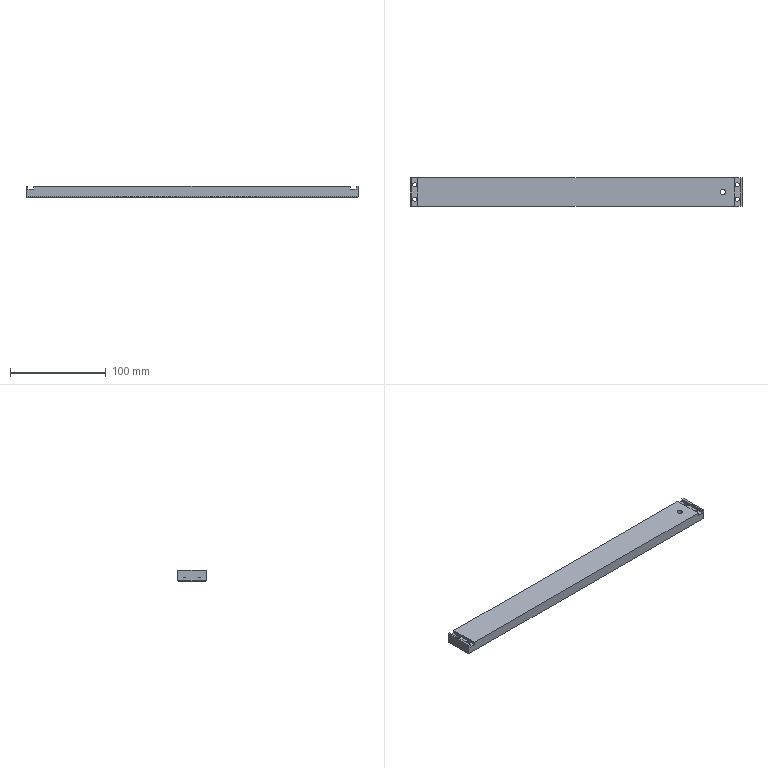CAM job | NX | 3-axis milling, drilling | part box 346 x 30 x 11.5 mm | stock box 351 x 35 x 15 mm
Tools:
number,name,description,diameter,corner_radius,flute_length,length,flutes
4,D4,平底铣刀-粗,4.0,0.0,25.0,75.0,2
9,D10,平底铣刀-粗,10.0,0.0,35.0,75.0,2
11,D4-J,平底铣刀-精,4.0,0.0,50.0,75.0,2
7,D6-J,平底铣刀-精,6.0,0.0,25.0,75.0,2
1,D80R0.8飞刀,圆鼻刀-粗,80.0,0.8,50.0,75.0,2
1,D80R0.8飞刀-J,圆鼻刀-精,80.0,0.8,50.0,75.0,2
2,D6倒角刀,倒角刀,6.0,0.0,3.0,25.0,2
11,ZT4.5,钻头,4.5,0.0,35.0,50.0,2
17,ZT5.5,钻头,5.5,0.0,35.0,50.0,2
Operations:
program,operation,operation_type,tool,method,geometry_group,spindle_rpm,surface_speed,feed_per_tooth,feed_cut,feed_plunge,cut_length_mm,path_length_mm,cut_time_min,machine_time_min
B,底壁铣飞面一刀开粗_COPY,VolumeBased25DMillingOperation,D80R0.8飞刀,分层开粗-切深K-步距G,W-B,2800.0,703.696,0.5357,3000.0,100.0,2725.164,5259.185,0.9084,1.162
B,底壁铣飞面一刀精光_COPY,VolumeBased25DMillingOperation,D80R0.8飞刀-J,侧刃精光-切深K-步距G,W-B,4000.0,1005.28,0.125,1000.0,100.0,453.998,549.998,0.454,0.4636
B,底壁铣分层开粗-中_COPY,VolumeBased25DMillingOperation,D4,分层开粗-切深K-步距G,W-B,8000.0,100.528,0.125,2000.0,100.0,1626.4,2005.684,0.8132,0.8511
B,平面去毛刺6X45L_COPY,SurfaceContour,D6倒角刀,爬面_倒角-切深0-步距G,W-B,6500.0,122.519,0.1154,1500.0,100.0,892.646,1870.716,0.5951,0.6929
B,底壁铣精光侧面-中-选底面_COPY,VolumeBased25DMillingOperation,D4-J,侧刃精光-切深K-步距G,W-B,8000.0,100.528,0.05,800.0,100.0,150.779,526.138,0.1885,0.226
A,顶面,FaceMilling,D80R0.8飞刀,侧刃精光-切深K-步距G,W-A,4500.0,1385.0,0.1667,1500.0,100.0,440.0,496.0,0.2933,0.2989
A,外形粗_2,VolumeBased25DMillingOperation,D10,METHOD,W-A,8000.0,251.327,0.375,6000.0,80.0,12546.214,12616.214,2.091,2.098
A,打点-深0.8,Operation,D6倒角刀,NONE,W-A,8000.0,150.796,0.0312,500.0,90.0,9.0,449.956,0.018,0.0621
A,沉头孔-钻孔0段,Operation,ZT4.5,NONE,W-A,2800.0,39.584,0.0179,100.0,90.0,51.408,531.884,0.5141,0.5621
A,通孔-5-6,Operation,ZT5.5,NONE,W-A,3000.0,51.836,0.025,150.0,90.0,16.152,92.305,0.1077,0.1153
A,铣孔开粗D4_1,CylinderMilling,D4,NONE,W-A,8000.0,100.531,0.075,1200.0,100.0,788.138,1408.138,0.6568,0.7188
A,等高螺旋爬面_COPY,ZLevelMilling,D4-J,等高爬面-切深K-步距G,W-A,7000.0,87.965,0.1429,2000.0,100.0,4015.858,4075.858,2.008,2.014
A,铣孔精光D4_1,CylinderMilling,D4-J,精光步距切深关,W-A,8000.0,100.531,0.0312,500.0,100.0,123.857,743.857,0.2477,0.3097
A,铣倒角_2,PlanarMilling,D6倒角刀,NONE,W-A,8000.0,150.796,0.0312,500.0,100.0,135.871,722.09,0.2717,0.3304
A,C0.3封闭铣廓倒角6X45L_COPY,PlanarMilling,D6倒角刀,爬面_倒角-切深0-步距G,W-A,7000.0,131.0,0.1071,1500.0,100.0,769.72,826.22,0.5131,0.5188
A,外形半精_2,VolumeBased25DMillingOperation,D6-J,METHOD,W-A,9000.0,169.646,0.0667,1200.0,100.0,775.766,857.766,0.6465,0.6547